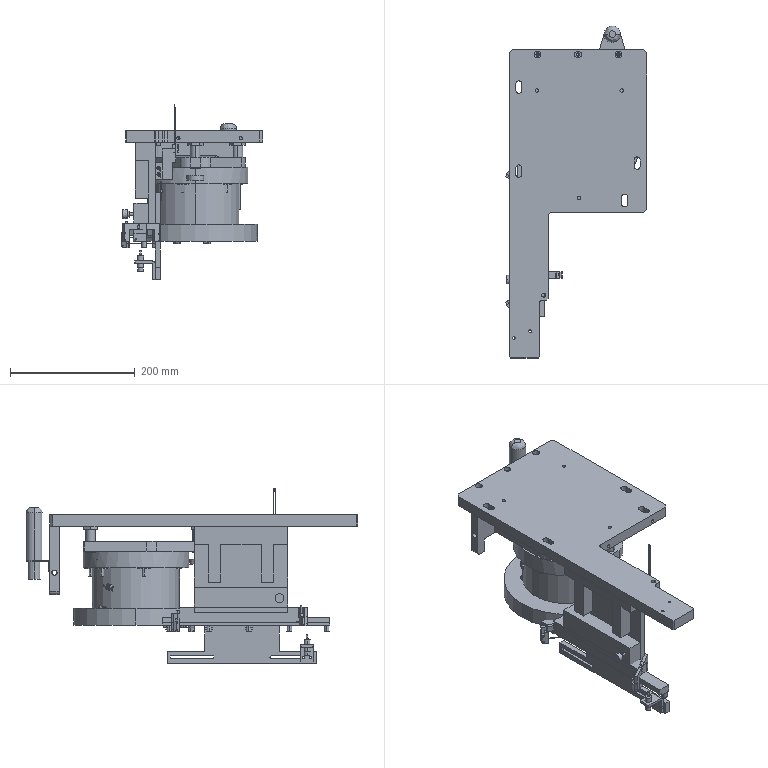Part | SolidWorks | features BaseBody 82, ICE 6, HoleWzd 4, Chamfer 2, Cut 1, Fillet 1 | 82 solids | 1903 faces | box 226.504 x 533.25 x 281.45 mm | volume 5326781 mm3 | plane 896 | cylinder 625 | cone 294 | spline 88 | commonest cylinder face diameters 10 x70 6 x66 2.5 x56 3.5 x42 5.5 x38 4 x32